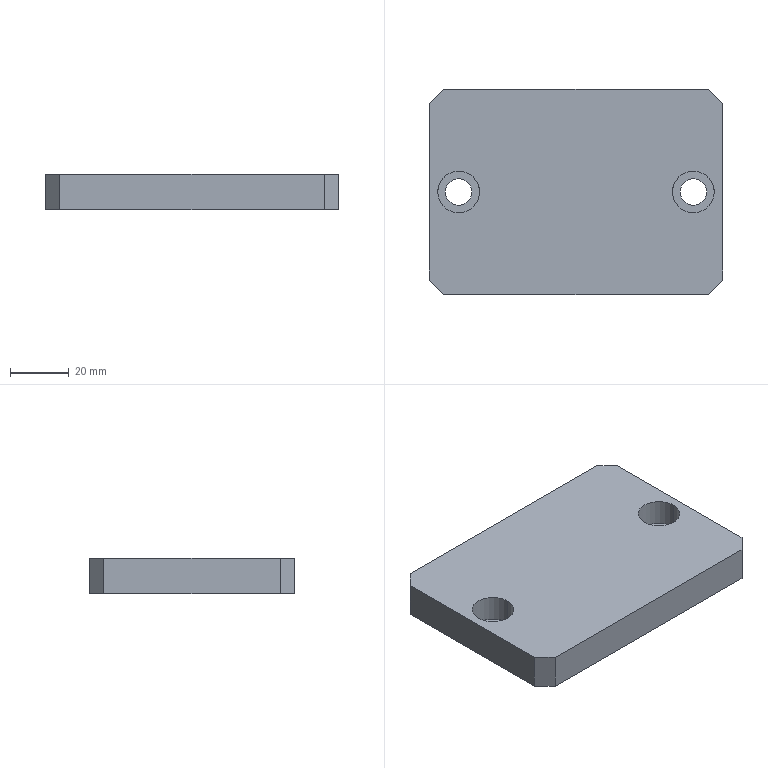Part | Creo | 1 solid | 20 faces | box 100 x 70 x 12 mm | volume 80148 mm3 | plane 12 | cylinder 8 | commonest cylinder face diameters 9 x4 14.25 x4
STEP:
#1=CARTESIAN_POINT('',(0.,0.,0.));
#2=DIRECTION('',(0.,0.,1.));
#3=DIRECTION('',(1.,0.,0.));
#4=AXIS2_PLACEMENT_3D('',#1,#2,#3);
#5=CARTESIAN_POINT('',(264.476,-389.127,-37.441));
#6=VERTEX_POINT('',#5);
#7=CARTESIAN_POINT('',(278.726,-389.127,-37.441));
#8=VERTEX_POINT('',#7);
#9=CARTESIAN_POINT('',(271.601,-389.127,-37.441));
#10=DIRECTION('',(0.,0.,1.));
#11=DIRECTION('',(-1.,0.,0.));
#12=AXIS2_PLACEMENT_3D('',#9,#10,#11);
#13=CIRCLE('',#12,7.125);
#14=EDGE_CURVE('',#6,#8,#13,.T.);
#15=ORIENTED_EDGE('',*,*,#14,.F.);
#16=CARTESIAN_POINT('',(271.601,-389.127,-37.441));
#17=DIRECTION('',(0.,0.,1.));
#18=DIRECTION('',(1.,0.,0.));
#19=AXIS2_PLACEMENT_3D('',#16,#17,#18);
#20=CIRCLE('',#19,7.125);
#21=EDGE_CURVE('',#8,#6,#20,.T.);
#22=ORIENTED_EDGE('',*,*,#21,.F.);
#23=EDGE_LOOP('',(#15,#22));
#24=FACE_OUTER_BOUND('',#23,.F.);
#25=CARTESIAN_POINT('',(276.101,-389.127,-37.441));
#26=VERTEX_POINT('',#25);
#27=CARTESIAN_POINT('',(267.101,-389.127,-37.441));
#28=VERTEX_POINT('',#27);
#29=CARTESIAN_POINT('',(271.601,-389.127,-37.441));
#30=DIRECTION('',(0.,0.,-1.));
#31=DIRECTION('',(1.,0.,0.));
#32=AXIS2_PLACEMENT_3D('',#29,#30,#31);
#33=CIRCLE('',#32,4.5);
#34=EDGE_CURVE('',#26,#28,#33,.T.);
#35=ORIENTED_EDGE('',*,*,#34,.F.);
#36=CARTESIAN_POINT('',(271.601,-389.127,-37.441));
#37=DIRECTION('',(0.,0.,-1.));
#38=DIRECTION('',(-1.,0.,0.));
#39=AXIS2_PLACEMENT_3D('',#36,#37,#38);
#40=CIRCLE('',#39,4.5);
#41=EDGE_CURVE('',#28,#26,#40,.T.);
#42=ORIENTED_EDGE('',*,*,#41,.F.);
#43=EDGE_LOOP('',(#35,#42));
#44=FACE_BOUND('',#43,.F.);
#45=CARTESIAN_POINT('',(271.601,-389.127,-37.441));
#46=DIRECTION('',(0.,0.,-1.));
#47=DIRECTION('',(-1.,0.,0.));
#48=AXIS2_PLACEMENT_3D('',#45,#46,#47);
#49=PLANE('',#48);
#50=ADVANCED_FACE('',(#24,#44),#49,.F.);
#51=CARTESIAN_POINT('',(267.101,-389.127,-40.441));
#52=VERTEX_POINT('',#51);
#53=CARTESIAN_POINT('',(276.101,-389.127,-40.441));
#54=VERTEX_POINT('',#53);
#55=CARTESIAN_POINT('',(271.601,-389.127,-40.441));
#56=DIRECTION('',(0.,0.,1.));
#57=DIRECTION('',(-1.,0.,0.));
#58=AXIS2_PLACEMENT_3D('',#55,#56,#57);
#59=CIRCLE('',#58,4.5);
#60=EDGE_CURVE('',#52,#54,#59,.T.);
#61=ORIENTED_EDGE('',*,*,#60,.T.);
#62=CARTESIAN_POINT('',(276.101,-389.127,-37.441));
#63=DIRECTION('',(0.,0.,-1.));
#64=VECTOR('',#63,3.);
#65=LINE('',#62,#64);
#66=EDGE_CURVE('',#26,#54,#65,.T.);
#67=ORIENTED_EDGE('',*,*,#66,.F.);
#68=ORIENTED_EDGE('',*,*,#34,.T.);
#69=CARTESIAN_POINT('',(267.101,-389.127,-37.441));
#70=DIRECTION('',(0.,0.,-1.));
#71=VECTOR('',#70,3.);
#72=LINE('',#69,#71);
#73=EDGE_CURVE('',#28,#52,#72,.T.);
#74=ORIENTED_EDGE('',*,*,#73,.T.);
#75=EDGE_LOOP('',(#61,#67,#68,#74));
#76=FACE_OUTER_BOUND('',#75,.F.);
#77=CARTESIAN_POINT('',(271.601,-389.127,-37.441));
#78=DIRECTION('',(0.,0.,-1.));
#79=DIRECTION('',(-1.,0.,0.));
#80=AXIS2_PLACEMENT_3D('',#77,#78,#79);
#81=CYLINDRICAL_SURFACE('',#80,4.5);
#82=ADVANCED_FACE('',(#76),#81,.F.);
#83=CARTESIAN_POINT('',(186.601,-424.127,-40.441));
#84=VERTEX_POINT('',#83);
#85=CARTESIAN_POINT('',(276.601,-424.127,-40.441));
#86=VERTEX_POINT('',#85);
#87=CARTESIAN_POINT('',(186.601,-424.127,-40.441));
#88=DIRECTION('',(1.,0.,0.));
#89=VECTOR('',#88,90.);
#90=LINE('',#87,#89);
#91=EDGE_CURVE('',#84,#86,#90,.T.);
#92=ORIENTED_EDGE('',*,*,#91,.T.);
#93=CARTESIAN_POINT('',(281.601,-419.127,-40.441));
#94=VERTEX_POINT('',#93);
#95=CARTESIAN_POINT('',(281.601,-419.127,-40.441));
#96=DIRECTION('',(-0.7071,-0.7071,0.));
#97=VECTOR('',#96,7.071);
#98=LINE('',#95,#97);
#99=EDGE_CURVE('',#94,#86,#98,.T.);
#100=ORIENTED_EDGE('',*,*,#99,.F.);
#101=CARTESIAN_POINT('',(281.601,-359.127,-40.441));
#102=VERTEX_POINT('',#101);
#103=CARTESIAN_POINT('',(281.601,-419.127,-40.441));
#104=DIRECTION('',(0.,1.,0.));
#105=VECTOR('',#104,60.);
#106=LINE('',#103,#105);
#107=EDGE_CURVE('',#94,#102,#106,.T.);
#108=ORIENTED_EDGE('',*,*,#107,.T.);
#109=CARTESIAN_POINT('',(276.601,-354.127,-40.441));
#110=VERTEX_POINT('',#109);
#111=CARTESIAN_POINT('',(276.601,-354.127,-40.441));
#112=DIRECTION('',(0.7071,-0.7071,0.));
#113=VECTOR('',#112,7.071);
#114=LINE('',#111,#113);
#115=EDGE_CURVE('',#110,#102,#114,.T.);
#116=ORIENTED_EDGE('',*,*,#115,.F.);
#117=CARTESIAN_POINT('',(186.601,-354.127,-40.441));
#118=VERTEX_POINT('',#117);
#119=CARTESIAN_POINT('',(276.601,-354.127,-40.441));
#120=DIRECTION('',(-1.,0.,0.));
#121=VECTOR('',#120,90.);
#122=LINE('',#119,#121);
#123=EDGE_CURVE('',#110,#118,#122,.T.);
#124=ORIENTED_EDGE('',*,*,#123,.T.);
#125=CARTESIAN_POINT('',(181.601,-359.127,-40.441));
#126=VERTEX_POINT('',#125);
#127=CARTESIAN_POINT('',(181.601,-359.127,-40.441));
#128=DIRECTION('',(0.7071,0.7071,0.));
#129=VECTOR('',#128,7.071);
#130=LINE('',#127,#129);
#131=EDGE_CURVE('',#126,#118,#130,.T.);
#132=ORIENTED_EDGE('',*,*,#131,.F.);
#133=CARTESIAN_POINT('',(181.601,-419.127,-40.441));
#134=VERTEX_POINT('',#133);
#135=CARTESIAN_POINT('',(181.601,-359.127,-40.441));
#136=DIRECTION('',(0.,-1.,0.));
#137=VECTOR('',#136,60.);
#138=LINE('',#135,#137);
#139=EDGE_CURVE('',#126,#134,#138,.T.);
#140=ORIENTED_EDGE('',*,*,#139,.T.);
#141=CARTESIAN_POINT('',(186.601,-424.127,-40.441));
#142=DIRECTION('',(-0.7071,0.7071,0.));
#143=VECTOR('',#142,7.071);
#144=LINE('',#141,#143);
#145=EDGE_CURVE('',#84,#134,#144,.T.);
#146=ORIENTED_EDGE('',*,*,#145,.F.);
#147=EDGE_LOOP('',(#92,#100,#108,#116,#124,#132,#140,#146));
#148=FACE_OUTER_BOUND('',#147,.F.);
#149=CARTESIAN_POINT('',(196.101,-389.127,-40.441));
#150=VERTEX_POINT('',#149);
#151=CARTESIAN_POINT('',(187.101,-389.127,-40.441));
#152=VERTEX_POINT('',#151);
#153=CARTESIAN_POINT('',(191.601,-389.127,-40.441));
#154=DIRECTION('',(0.,0.,1.));
#155=DIRECTION('',(1.,0.,0.));
#156=AXIS2_PLACEMENT_3D('',#153,#154,#155);
#157=CIRCLE('',#156,4.5);
#158=EDGE_CURVE('',#150,#152,#157,.T.);
#159=ORIENTED_EDGE('',*,*,#158,.F.);
#160=CARTESIAN_POINT('',(191.601,-389.127,-40.441));
#161=DIRECTION('',(0.,0.,1.));
#162=DIRECTION('',(-1.,0.,0.));
#163=AXIS2_PLACEMENT_3D('',#160,#161,#162);
#164=CIRCLE('',#163,4.5);
#165=EDGE_CURVE('',#152,#150,#164,.T.);
#166=ORIENTED_EDGE('',*,*,#165,.F.);
#167=EDGE_LOOP('',(#159,#166));
#168=FACE_BOUND('',#167,.F.);
#169=CARTESIAN_POINT('',(271.601,-389.127,-40.441));
#170=DIRECTION('',(0.,0.,1.));
#171=DIRECTION('',(1.,0.,0.));
#172=AXIS2_PLACEMENT_3D('',#169,#170,#171);
#173=CIRCLE('',#172,4.5);
#174=EDGE_CURVE('',#54,#52,#173,.T.);
#175=ORIENTED_EDGE('',*,*,#174,.F.);
#176=ORIENTED_EDGE('',*,*,#60,.F.);
#177=EDGE_LOOP('',(#175,#176));
#178=FACE_BOUND('',#177,.F.);
#179=CARTESIAN_POINT('',(181.601,-354.127,-40.441));
#180=DIRECTION('',(0.,0.,-1.));
#181=DIRECTION('',(-1.,0.,0.));
#182=AXIS2_PLACEMENT_3D('',#179,#180,#181);
#183=PLANE('',#182);
#184=ADVANCED_FACE('',(#148,#168,#178),#183,.T.);
#185=ORIENTED_EDGE('',*,*,#174,.T.);
#186=ORIENTED_EDGE('',*,*,#73,.F.);
#187=ORIENTED_EDGE('',*,*,#41,.T.);
#188=ORIENTED_EDGE('',*,*,#66,.T.);
#189=EDGE_LOOP('',(#185,#186,#187,#188));
#190=FACE_OUTER_BOUND('',#189,.F.);
#191=CARTESIAN_POINT('',(271.601,-389.127,-37.441));
#192=DIRECTION('',(0.,0.,-1.));
#193=DIRECTION('',(-1.,0.,0.));
#194=AXIS2_PLACEMENT_3D('',#191,#192,#193);
#195=CYLINDRICAL_SURFACE('',#194,4.5);
#196=ADVANCED_FACE('',(#190),#195,.F.);
#197=ORIENTED_EDGE('',*,*,#158,.T.);
#198=CARTESIAN_POINT('',(187.101,-389.127,-37.441));
#199=VERTEX_POINT('',#198);
#200=CARTESIAN_POINT('',(187.101,-389.127,-37.441));
#201=DIRECTION('',(0.,0.,-1.));
#202=VECTOR('',#201,3.);
#203=LINE('',#200,#202);
#204=EDGE_CURVE('',#199,#152,#203,.T.);
#205=ORIENTED_EDGE('',*,*,#204,.F.);
#206=CARTESIAN_POINT('',(196.101,-389.127,-37.441));
#207=VERTEX_POINT('',#206);
#208=CARTESIAN_POINT('',(191.601,-389.127,-37.441));
#209=DIRECTION('',(0.,0.,-1.));
#210=DIRECTION('',(-1.,0.,0.));
#211=AXIS2_PLACEMENT_3D('',#208,#209,#210);
#212=CIRCLE('',#211,4.5);
#213=EDGE_CURVE('',#199,#207,#212,.T.);
#214=ORIENTED_EDGE('',*,*,#213,.T.);
#215=CARTESIAN_POINT('',(196.101,-389.127,-37.441));
#216=DIRECTION('',(0.,0.,-1.));
#217=VECTOR('',#216,3.);
#218=LINE('',#215,#217);
#219=EDGE_CURVE('',#207,#150,#218,.T.);
#220=ORIENTED_EDGE('',*,*,#219,.T.);
#221=EDGE_LOOP('',(#197,#205,#214,#220));
#222=FACE_OUTER_BOUND('',#221,.F.);
#223=CARTESIAN_POINT('',(191.601,-389.127,-37.441));
#224=DIRECTION('',(0.,0.,-1.));
#225=DIRECTION('',(-1.,0.,0.));
#226=AXIS2_PLACEMENT_3D('',#223,#224,#225);
#227=CYLINDRICAL_SURFACE('',#226,4.5);
#228=ADVANCED_FACE('',(#222),#227,.F.);
#229=ORIENTED_EDGE('',*,*,#165,.T.);
#230=ORIENTED_EDGE('',*,*,#219,.F.);
#231=CARTESIAN_POINT('',(191.601,-389.127,-37.441));
#232=DIRECTION('',(0.,0.,-1.));
#233=DIRECTION('',(1.,0.,0.));
#234=AXIS2_PLACEMENT_3D('',#231,#232,#233);
#235=CIRCLE('',#234,4.5);
#236=EDGE_CURVE('',#207,#199,#235,.T.);
#237=ORIENTED_EDGE('',*,*,#236,.T.);
#238=ORIENTED_EDGE('',*,*,#204,.T.);
#239=EDGE_LOOP('',(#229,#230,#237,#238));
#240=FACE_OUTER_BOUND('',#239,.F.);
#241=CARTESIAN_POINT('',(191.601,-389.127,-37.441));
#242=DIRECTION('',(0.,0.,-1.));
#243=DIRECTION('',(-1.,0.,0.));
#244=AXIS2_PLACEMENT_3D('',#241,#242,#243);
#245=CYLINDRICAL_SURFACE('',#244,4.5);
#246=ADVANCED_FACE('',(#240),#245,.F.);
#247=CARTESIAN_POINT('',(184.476,-389.127,-37.441));
#248=VERTEX_POINT('',#247);
#249=CARTESIAN_POINT('',(198.726,-389.127,-37.441));
#250=VERTEX_POINT('',#249);
#251=CARTESIAN_POINT('',(191.601,-389.127,-37.441));
#252=DIRECTION('',(0.,0.,1.));
#253=DIRECTION('',(-1.,0.,0.));
#254=AXIS2_PLACEMENT_3D('',#251,#252,#253);
#255=CIRCLE('',#254,7.125);
#256=EDGE_CURVE('',#248,#250,#255,.T.);
#257=ORIENTED_EDGE('',*,*,#256,.F.);
#258=CARTESIAN_POINT('',(191.601,-389.127,-37.441));
#259=DIRECTION('',(0.,0.,1.));
#260=DIRECTION('',(1.,0.,0.));
#261=AXIS2_PLACEMENT_3D('',#258,#259,#260);
#262=CIRCLE('',#261,7.125);
#263=EDGE_CURVE('',#250,#248,#262,.T.);
#264=ORIENTED_EDGE('',*,*,#263,.F.);
#265=EDGE_LOOP('',(#257,#264));
#266=FACE_OUTER_BOUND('',#265,.F.);
#267=ORIENTED_EDGE('',*,*,#236,.F.);
#268=ORIENTED_EDGE('',*,*,#213,.F.);
#269=EDGE_LOOP('',(#267,#268));
#270=FACE_BOUND('',#269,.F.);
#271=CARTESIAN_POINT('',(191.601,-389.127,-37.441));
#272=DIRECTION('',(0.,0.,-1.));
#273=DIRECTION('',(-1.,0.,0.));
#274=AXIS2_PLACEMENT_3D('',#271,#272,#273);
#275=PLANE('',#274);
#276=ADVANCED_FACE('',(#266,#270),#275,.F.);
#277=CARTESIAN_POINT('',(198.726,-389.127,-28.441));
#278=VERTEX_POINT('',#277);
#279=CARTESIAN_POINT('',(184.476,-389.127,-28.441));
#280=VERTEX_POINT('',#279);
#281=CARTESIAN_POINT('',(191.601,-389.127,-28.441));
#282=DIRECTION('',(0.,0.,-1.));
#283=DIRECTION('',(1.,0.,0.));
#284=AXIS2_PLACEMENT_3D('',#281,#282,#283);
#285=CIRCLE('',#284,7.125);
#286=EDGE_CURVE('',#278,#280,#285,.T.);
#287=ORIENTED_EDGE('',*,*,#286,.T.);
#288=CARTESIAN_POINT('',(184.476,-389.127,-37.441));
#289=DIRECTION('',(0.,0.,1.));
#290=VECTOR('',#289,9.);
#291=LINE('',#288,#290);
#292=EDGE_CURVE('',#248,#280,#291,.T.);
#293=ORIENTED_EDGE('',*,*,#292,.F.);
#294=ORIENTED_EDGE('',*,*,#256,.T.);
#295=CARTESIAN_POINT('',(198.726,-389.127,-37.441));
#296=DIRECTION('',(0.,0.,1.));
#297=VECTOR('',#296,9.);
#298=LINE('',#295,#297);
#299=EDGE_CURVE('',#250,#278,#298,.T.);
#300=ORIENTED_EDGE('',*,*,#299,.T.);
#301=EDGE_LOOP('',(#287,#293,#294,#300));
#302=FACE_OUTER_BOUND('',#301,.F.);
#303=CARTESIAN_POINT('',(191.601,-389.127,-37.441));
#304=DIRECTION('',(0.,0.,1.));
#305=DIRECTION('',(1.,0.,0.));
#306=AXIS2_PLACEMENT_3D('',#303,#304,#305);
#307=CYLINDRICAL_SURFACE('',#306,7.125);
#308=ADVANCED_FACE('',(#302),#307,.F.);
#309=CARTESIAN_POINT('',(181.601,-359.127,-28.441));
#310=VERTEX_POINT('',#309);
#311=CARTESIAN_POINT('',(181.601,-419.127,-28.441));
#312=VERTEX_POINT('',#311);
#313=CARTESIAN_POINT('',(181.601,-359.127,-28.441));
#314=DIRECTION('',(0.,-1.,0.));
#315=VECTOR('',#314,60.);
#316=LINE('',#313,#315);
#317=EDGE_CURVE('',#310,#312,#316,.T.);
#318=ORIENTED_EDGE('',*,*,#317,.F.);
#319=CARTESIAN_POINT('',(186.601,-354.127,-28.441));
#320=VERTEX_POINT('',#319);
#321=CARTESIAN_POINT('',(186.601,-354.127,-28.441));
#322=DIRECTION('',(-0.7071,-0.7071,0.));
#323=VECTOR('',#322,7.071);
#324=LINE('',#321,#323);
#325=EDGE_CURVE('',#320,#310,#324,.T.);
#326=ORIENTED_EDGE('',*,*,#325,.F.);
#327=CARTESIAN_POINT('',(276.601,-354.127,-28.441));
#328=VERTEX_POINT('',#327);
#329=CARTESIAN_POINT('',(276.601,-354.127,-28.441));
#330=DIRECTION('',(-1.,0.,0.));
#331=VECTOR('',#330,90.);
#332=LINE('',#329,#331);
#333=EDGE_CURVE('',#328,#320,#332,.T.);
#334=ORIENTED_EDGE('',*,*,#333,.F.);
#335=CARTESIAN_POINT('',(281.601,-359.127,-28.441));
#336=VERTEX_POINT('',#335);
#337=CARTESIAN_POINT('',(281.601,-359.127,-28.441));
#338=DIRECTION('',(-0.7071,0.7071,0.));
#339=VECTOR('',#338,7.071);
#340=LINE('',#337,#339);
#341=EDGE_CURVE('',#336,#328,#340,.T.);
#342=ORIENTED_EDGE('',*,*,#341,.F.);
#343=CARTESIAN_POINT('',(281.601,-419.127,-28.441));
#344=VERTEX_POINT('',#343);
#345=CARTESIAN_POINT('',(281.601,-419.127,-28.441));
#346=DIRECTION('',(0.,1.,0.));
#347=VECTOR('',#346,60.);
#348=LINE('',#345,#347);
#349=EDGE_CURVE('',#344,#336,#348,.T.);
#350=ORIENTED_EDGE('',*,*,#349,.F.);
#351=CARTESIAN_POINT('',(276.601,-424.127,-28.441));
#352=VERTEX_POINT('',#351);
#353=CARTESIAN_POINT('',(276.601,-424.127,-28.441));
#354=DIRECTION('',(0.7071,0.7071,0.));
#355=VECTOR('',#354,7.071);
#356=LINE('',#353,#355);
#357=EDGE_CURVE('',#352,#344,#356,.T.);
#358=ORIENTED_EDGE('',*,*,#357,.F.);
#359=CARTESIAN_POINT('',(186.601,-424.127,-28.441));
#360=VERTEX_POINT('',#359);
#361=CARTESIAN_POINT('',(186.601,-424.127,-28.441));
#362=DIRECTION('',(1.,0.,0.));
#363=VECTOR('',#362,90.);
#364=LINE('',#361,#363);
#365=EDGE_CURVE('',#360,#352,#364,.T.);
#366=ORIENTED_EDGE('',*,*,#365,.F.);
#367=CARTESIAN_POINT('',(181.601,-419.127,-28.441));
#368=DIRECTION('',(0.7071,-0.7071,0.));
#369=VECTOR('',#368,7.071);
#370=LINE('',#367,#369);
#371=EDGE_CURVE('',#312,#360,#370,.T.);
#372=ORIENTED_EDGE('',*,*,#371,.F.);
#373=EDGE_LOOP('',(#318,#326,#334,#342,#350,#358,#366,#372));
#374=FACE_OUTER_BOUND('',#373,.F.);
#375=CARTESIAN_POINT('',(191.601,-389.127,-28.441));
#376=DIRECTION('',(0.,0.,-1.));
#377=DIRECTION('',(-1.,0.,0.));
#378=AXIS2_PLACEMENT_3D('',#375,#376,#377);
#379=CIRCLE('',#378,7.125);
#380=EDGE_CURVE('',#280,#278,#379,.T.);
#381=ORIENTED_EDGE('',*,*,#380,.F.);
#382=ORIENTED_EDGE('',*,*,#286,.F.);
#383=EDGE_LOOP('',(#381,#382));
#384=FACE_BOUND('',#383,.F.);
#385=CARTESIAN_POINT('',(264.476,-389.127,-28.441));
#386=VERTEX_POINT('',#385);
#387=CARTESIAN_POINT('',(278.726,-389.127,-28.441));
#388=VERTEX_POINT('',#387);
#389=CARTESIAN_POINT('',(271.601,-389.127,-28.441));
#390=DIRECTION('',(0.,0.,-1.));
#391=DIRECTION('',(-1.,0.,0.));
#392=AXIS2_PLACEMENT_3D('',#389,#390,#391);
#393=CIRCLE('',#392,7.125);
#394=EDGE_CURVE('',#386,#388,#393,.T.);
#395=ORIENTED_EDGE('',*,*,#394,.F.);
#396=CARTESIAN_POINT('',(271.601,-389.127,-28.441));
#397=DIRECTION('',(0.,0.,-1.));
#398=DIRECTION('',(1.,0.,0.));
#399=AXIS2_PLACEMENT_3D('',#396,#397,#398);
#400=CIRCLE('',#399,7.125);
#401=EDGE_CURVE('',#388,#386,#400,.T.);
#402=ORIENTED_EDGE('',*,*,#401,.F.);
#403=EDGE_LOOP('',(#395,#402));
#404=FACE_BOUND('',#403,.F.);
#405=CARTESIAN_POINT('',(181.601,-354.127,-28.441));
#406=DIRECTION('',(0.,0.,-1.));
#407=DIRECTION('',(-1.,0.,0.));
#408=AXIS2_PLACEMENT_3D('',#405,#406,#407);
#409=PLANE('',#408);
#410=ADVANCED_FACE('',(#374,#384,#404),#409,.F.);
#411=ORIENTED_EDGE('',*,*,#380,.T.);
#412=ORIENTED_EDGE('',*,*,#299,.F.);
#413=ORIENTED_EDGE('',*,*,#263,.T.);
#414=ORIENTED_EDGE('',*,*,#292,.T.);
#415=EDGE_LOOP('',(#411,#412,#413,#414));
#416=FACE_OUTER_BOUND('',#415,.F.);
#417=CARTESIAN_POINT('',(191.601,-389.127,-37.441));
#418=DIRECTION('',(0.,0.,1.));
#419=DIRECTION('',(1.,0.,0.));
#420=AXIS2_PLACEMENT_3D('',#417,#418,#419);
#421=CYLINDRICAL_SURFACE('',#420,7.125);
#422=ADVANCED_FACE('',(#416),#421,.F.);
#423=ORIENTED_EDGE('',*,*,#139,.F.);
#424=CARTESIAN_POINT('',(181.601,-359.127,-40.441));
#425=DIRECTION('',(0.,0.,1.));
#426=VECTOR('',#425,12.);
#427=LINE('',#424,#426);
#428=EDGE_CURVE('',#126,#310,#427,.T.);
#429=ORIENTED_EDGE('',*,*,#428,.T.);
#430=ORIENTED_EDGE('',*,*,#317,.T.);
#431=CARTESIAN_POINT('',(181.601,-419.127,-28.441));
#432=DIRECTION('',(0.,0.,-1.));
#433=VECTOR('',#432,12.);
#434=LINE('',#431,#433);
#435=EDGE_CURVE('',#312,#134,#434,.T.);
#436=ORIENTED_EDGE('',*,*,#435,.T.);
#437=EDGE_LOOP('',(#423,#429,#430,#436));
#438=FACE_OUTER_BOUND('',#437,.F.);
#439=CARTESIAN_POINT('',(181.601,-424.127,-40.441));
#440=DIRECTION('',(1.,0.,0.));
#441=DIRECTION('',(0.,0.,-1.));
#442=AXIS2_PLACEMENT_3D('',#439,#440,#441);
#443=PLANE('',#442);
#444=ADVANCED_FACE('',(#438),#443,.F.);
#445=ORIENTED_EDGE('',*,*,#131,.T.);
#446=CARTESIAN_POINT('',(186.601,-354.127,-28.441));
#447=DIRECTION('',(0.,0.,-1.));
#448=VECTOR('',#447,12.);
#449=LINE('',#446,#448);
#450=EDGE_CURVE('',#320,#118,#449,.T.);
#451=ORIENTED_EDGE('',*,*,#450,.F.);
#452=ORIENTED_EDGE('',*,*,#325,.T.);
#453=ORIENTED_EDGE('',*,*,#428,.F.);
#454=EDGE_LOOP('',(#445,#451,#452,#453));
#455=FACE_OUTER_BOUND('',#454,.F.);
#456=CARTESIAN_POINT('',(186.601,-354.127,-40.441));
#457=DIRECTION('',(0.7071,-0.7071,0.));
#458=DIRECTION('',(0.7071,0.7071,0.));
#459=AXIS2_PLACEMENT_3D('',#456,#457,#458);
#460=PLANE('',#459);
#461=ADVANCED_FACE('',(#455),#460,.F.);
#462=ORIENTED_EDGE('',*,*,#123,.F.);
#463=CARTESIAN_POINT('',(276.601,-354.127,-40.441));
#464=DIRECTION('',(0.,0.,1.));
#465=VECTOR('',#464,12.);
#466=LINE('',#463,#465);
#467=EDGE_CURVE('',#110,#328,#466,.T.);
#468=ORIENTED_EDGE('',*,*,#467,.T.);
#469=ORIENTED_EDGE('',*,*,#333,.T.);
#470=ORIENTED_EDGE('',*,*,#450,.T.);
#471=EDGE_LOOP('',(#462,#468,#469,#470));
#472=FACE_OUTER_BOUND('',#471,.F.);
#473=CARTESIAN_POINT('',(181.601,-354.127,-40.441));
#474=DIRECTION('',(0.,-1.,0.));
#475=DIRECTION('',(0.,0.,-1.));
#476=AXIS2_PLACEMENT_3D('',#473,#474,#475);
#477=PLANE('',#476);
#478=ADVANCED_FACE('',(#472),#477,.F.);
#479=ORIENTED_EDGE('',*,*,#115,.T.);
#480=CARTESIAN_POINT('',(281.601,-359.127,-28.441));
#481=DIRECTION('',(0.,0.,-1.));
#482=VECTOR('',#481,12.);
#483=LINE('',#480,#482);
#484=EDGE_CURVE('',#336,#102,#483,.T.);
#485=ORIENTED_EDGE('',*,*,#484,.F.);
#486=ORIENTED_EDGE('',*,*,#341,.T.);
#487=ORIENTED_EDGE('',*,*,#467,.F.);
#488=EDGE_LOOP('',(#479,#485,#486,#487));
#489=FACE_OUTER_BOUND('',#488,.F.);
#490=CARTESIAN_POINT('',(281.601,-359.127,-40.441));
#491=DIRECTION('',(-0.7071,-0.7071,0.));
#492=DIRECTION('',(0.7071,-0.7071,0.));
#493=AXIS2_PLACEMENT_3D('',#490,#491,#492);
#494=PLANE('',#493);
#495=ADVANCED_FACE('',(#489),#494,.F.);
#496=ORIENTED_EDGE('',*,*,#349,.T.);
#497=ORIENTED_EDGE('',*,*,#484,.T.);
#498=ORIENTED_EDGE('',*,*,#107,.F.);
#499=CARTESIAN_POINT('',(281.601,-419.127,-40.441));
#500=DIRECTION('',(0.,0.,1.));
#501=VECTOR('',#500,12.);
#502=LINE('',#499,#501);
#503=EDGE_CURVE('',#94,#344,#502,.T.);
#504=ORIENTED_EDGE('',*,*,#503,.T.);
#505=EDGE_LOOP('',(#496,#497,#498,#504));
#506=FACE_OUTER_BOUND('',#505,.F.);
#507=CARTESIAN_POINT('',(281.601,-354.127,-40.441));
#508=DIRECTION('',(-1.,0.,0.));
#509=DIRECTION('',(0.,0.,1.));
#510=AXIS2_PLACEMENT_3D('',#507,#508,#509);
#511=PLANE('',#510);
#512=ADVANCED_FACE('',(#506),#511,.F.);
#513=ORIENTED_EDGE('',*,*,#99,.T.);
#514=CARTESIAN_POINT('',(276.601,-424.127,-28.441));
#515=DIRECTION('',(0.,0.,-1.));
#516=VECTOR('',#515,12.);
#517=LINE('',#514,#516);
#518=EDGE_CURVE('',#352,#86,#517,.T.);
#519=ORIENTED_EDGE('',*,*,#518,.F.);
#520=ORIENTED_EDGE('',*,*,#357,.T.);
#521=ORIENTED_EDGE('',*,*,#503,.F.);
#522=EDGE_LOOP('',(#513,#519,#520,#521));
#523=FACE_OUTER_BOUND('',#522,.F.);
#524=CARTESIAN_POINT('',(276.601,-424.127,-40.441));
#525=DIRECTION('',(-0.7071,0.7071,0.));
#526=DIRECTION('',(-0.7071,-0.7071,0.));
#527=AXIS2_PLACEMENT_3D('',#524,#525,#526);
#528=PLANE('',#527);
#529=ADVANCED_FACE('',(#523),#528,.F.);
#530=ORIENTED_EDGE('',*,*,#365,.T.);
#531=ORIENTED_EDGE('',*,*,#518,.T.);
#532=ORIENTED_EDGE('',*,*,#91,.F.);
#533=CARTESIAN_POINT('',(186.601,-424.127,-40.441));
#534=DIRECTION('',(0.,0.,1.));
#535=VECTOR('',#534,12.);
#536=LINE('',#533,#535);
#537=EDGE_CURVE('',#84,#360,#536,.T.);
#538=ORIENTED_EDGE('',*,*,#537,.T.);
#539=EDGE_LOOP('',(#530,#531,#532,#538));
#540=FACE_OUTER_BOUND('',#539,.F.);
#541=CARTESIAN_POINT('',(281.601,-424.127,-40.441));
#542=DIRECTION('',(0.,1.,0.));
#543=DIRECTION('',(0.,0.,1.));
#544=AXIS2_PLACEMENT_3D('',#541,#542,#543);
#545=PLANE('',#544);
#546=ADVANCED_FACE('',(#540),#545,.F.);
#547=ORIENTED_EDGE('',*,*,#145,.T.);
#548=ORIENTED_EDGE('',*,*,#435,.F.);
#549=ORIENTED_EDGE('',*,*,#371,.T.);
#550=ORIENTED_EDGE('',*,*,#537,.F.);
#551=EDGE_LOOP('',(#547,#548,#549,#550));
#552=FACE_OUTER_BOUND('',#551,.F.);
#553=CARTESIAN_POINT('',(181.601,-419.127,-40.441));
#554=DIRECTION('',(0.7071,0.7071,0.));
#555=DIRECTION('',(-0.7071,0.7071,0.));
#556=AXIS2_PLACEMENT_3D('',#553,#554,#555);
#557=PLANE('',#556);
#558=ADVANCED_FACE('',(#552),#557,.F.);
#559=ORIENTED_EDGE('',*,*,#394,.T.);
#560=CARTESIAN_POINT('',(278.726,-389.127,-37.441));
#561=DIRECTION('',(0.,0.,1.));
#562=VECTOR('',#561,9.);
#563=LINE('',#560,#562);
#564=EDGE_CURVE('',#8,#388,#563,.T.);
#565=ORIENTED_EDGE('',*,*,#564,.F.);
#566=ORIENTED_EDGE('',*,*,#21,.T.);
#567=CARTESIAN_POINT('',(264.476,-389.127,-37.441));
#568=DIRECTION('',(0.,0.,1.));
#569=VECTOR('',#568,9.);
#570=LINE('',#567,#569);
#571=EDGE_CURVE('',#6,#386,#570,.T.);
#572=ORIENTED_EDGE('',*,*,#571,.T.);
#573=EDGE_LOOP('',(#559,#565,#566,#572));
#574=FACE_OUTER_BOUND('',#573,.F.);
#575=CARTESIAN_POINT('',(271.601,-389.127,-37.441));
#576=DIRECTION('',(0.,0.,1.));
#577=DIRECTION('',(1.,0.,0.));
#578=AXIS2_PLACEMENT_3D('',#575,#576,#577);
#579=CYLINDRICAL_SURFACE('',#578,7.125);
#580=ADVANCED_FACE('',(#574),#579,.F.);
#581=ORIENTED_EDGE('',*,*,#401,.T.);
#582=ORIENTED_EDGE('',*,*,#571,.F.);
#583=ORIENTED_EDGE('',*,*,#14,.T.);
#584=ORIENTED_EDGE('',*,*,#564,.T.);
#585=EDGE_LOOP('',(#581,#582,#583,#584));
#586=FACE_OUTER_BOUND('',#585,.F.);
#587=CARTESIAN_POINT('',(271.601,-389.127,-37.441));
#588=DIRECTION('',(0.,0.,1.));
#589=DIRECTION('',(1.,0.,0.));
#590=AXIS2_PLACEMENT_3D('',#587,#588,#589);
#591=CYLINDRICAL_SURFACE('',#590,7.125);
#592=ADVANCED_FACE('',(#586),#591,.F.);
#593=CLOSED_SHELL('',(#50,#82,#184,#196,#228,#246,#276,#308,#410,#422,#444,#461,#478,#495,#512,#529,#546,#558,#580,#592));
#594=MANIFOLD_SOLID_BREP('',#593);
#595=(LENGTH_UNIT()NAMED_UNIT(*)SI_UNIT(.MILLI.,.METRE.));
#596=UNCERTAINTY_MEASURE_WITH_UNIT(LENGTH_MEASURE(0.01226),#595,'','');
#597=(NAMED_UNIT(*)PLANE_ANGLE_UNIT()SI_UNIT($,.RADIAN.));
#598=PLANE_ANGLE_MEASURE_WITH_UNIT(PLANE_ANGLE_MEASURE(0.01745),#597);
#599=(CONVERSION_BASED_UNIT('DEGREE',#598)NAMED_UNIT(*)PLANE_ANGLE_UNIT());
#600=(NAMED_UNIT(*)SI_UNIT($,.STERADIAN.)SOLID_ANGLE_UNIT());
#601=(GEOMETRIC_REPRESENTATION_CONTEXT(3)GLOBAL_UNCERTAINTY_ASSIGNED_CONTEXT((#596))GLOBAL_UNIT_ASSIGNED_CONTEXT((#595,#599,#600))REPRESENTATION_CONTEXT('',''));
#602=ADVANCED_BREP_SHAPE_REPRESENTATION('',(#4,#594),#601);